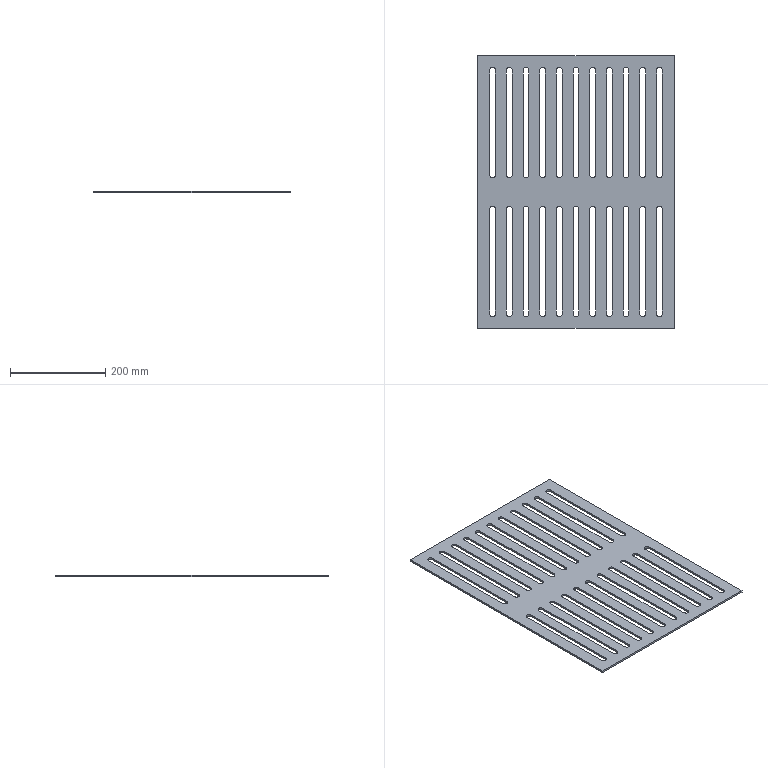Part | SolidWorks | features Extrusion 1, ICE 1 | 1 solid | 94 faces | box 413 x 572 x 4 mm | volume 702671 mm3 | plane 50 | cylinder 44 | commonest cylinder face diameters 12 x44